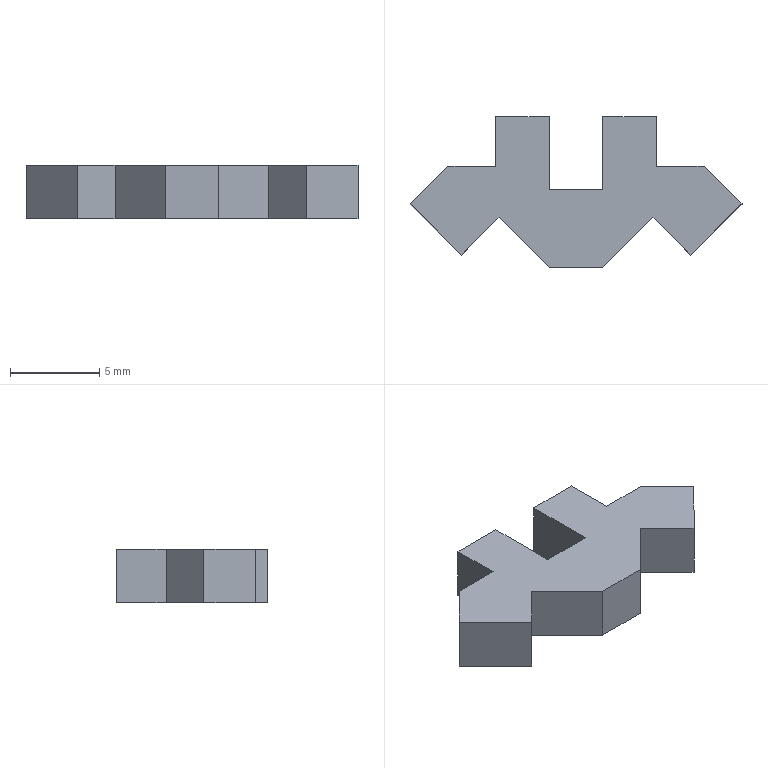Part | SolidWorks | features BaseBody 1 | 1 solid | 20 faces | box 18.567 x 8.438 x 3 mm | volume 257.816 mm3 | plane 20
STEP:
#1=CARTESIAN_POINT('',(-32.996,6.652,-1.5));
#2=VERTEX_POINT('',#1);
#3=CARTESIAN_POINT('',(-35.116,8.77,-1.5));
#4=VERTEX_POINT('',#3);
#5=CARTESIAN_POINT('',(-35.116,8.77,-1.5));
#6=DIRECTION('',(-0.7074,0.7068,0.));
#7=VECTOR('',#6,1000.);
#8=LINE('',#5,#7);
#9=EDGE_CURVE('',#2,#4,#8,.T.);
#10=ORIENTED_EDGE('',*,*,#9,.F.);
#11=CARTESIAN_POINT('',(-35.854,3.792,-1.5));
#12=VERTEX_POINT('',#11);
#13=CARTESIAN_POINT('',(-32.996,6.652,-1.5));
#14=DIRECTION('',(0.7068,0.7074,0.));
#15=VECTOR('',#14,1000.);
#16=LINE('',#13,#15);
#17=EDGE_CURVE('',#12,#2,#16,.T.);
#18=ORIENTED_EDGE('',*,*,#17,.F.);
#19=CARTESIAN_POINT('',(-37.974,5.912,-1.5));
#20=VERTEX_POINT('',#19);
#21=CARTESIAN_POINT('',(-35.854,3.792,-1.5));
#22=DIRECTION('',(0.707,-0.7072,0.));
#23=VECTOR('',#22,1000.);
#24=LINE('',#21,#23);
#25=EDGE_CURVE('',#20,#12,#24,.T.);
#26=ORIENTED_EDGE('',*,*,#25,.F.);
#27=CARTESIAN_POINT('',(-40.782,3.103,-1.5));
#28=VERTEX_POINT('',#27);
#29=CARTESIAN_POINT('',(-37.974,5.912,-1.5));
#30=DIRECTION('',(0.707,0.7072,0.));
#31=VECTOR('',#30,1000.);
#32=LINE('',#29,#31);
#33=EDGE_CURVE('',#28,#20,#32,.T.);
#34=ORIENTED_EDGE('',*,*,#33,.F.);
#35=CARTESIAN_POINT('',(-43.778,3.103,-1.5));
#36=VERTEX_POINT('',#35);
#37=CARTESIAN_POINT('',(-40.782,3.103,-1.5));
#38=DIRECTION('',(1.,0.,0.));
#39=VECTOR('',#38,1000.);
#40=LINE('',#37,#39);
#41=EDGE_CURVE('',#36,#28,#40,.T.);
#42=ORIENTED_EDGE('',*,*,#41,.F.);
#43=CARTESIAN_POINT('',(-46.585,5.913,-1.5));
#44=VERTEX_POINT('',#43);
#45=CARTESIAN_POINT('',(-43.778,3.103,-1.5));
#46=DIRECTION('',(0.7067,-0.7075,0.));
#47=VECTOR('',#46,1000.);
#48=LINE('',#45,#47);
#49=EDGE_CURVE('',#44,#36,#48,.T.);
#50=ORIENTED_EDGE('',*,*,#49,.F.);
#51=CARTESIAN_POINT('',(-48.705,3.792,-1.5));
#52=VERTEX_POINT('',#51);
#53=CARTESIAN_POINT('',(-46.585,5.913,-1.5));
#54=DIRECTION('',(0.707,0.7072,0.));
#55=VECTOR('',#54,1000.);
#56=LINE('',#53,#55);
#57=EDGE_CURVE('',#52,#44,#56,.T.);
#58=ORIENTED_EDGE('',*,*,#57,.F.);
#59=CARTESIAN_POINT('',(-51.564,6.652,-1.5));
#60=VERTEX_POINT('',#59);
#61=CARTESIAN_POINT('',(-48.705,3.792,-1.5));
#62=DIRECTION('',(0.7068,-0.7074,0.));
#63=VECTOR('',#62,1000.);
#64=LINE('',#61,#63);
#65=EDGE_CURVE('',#60,#52,#64,.T.);
#66=ORIENTED_EDGE('',*,*,#65,.F.);
#67=CARTESIAN_POINT('',(-49.444,8.77,-1.5));
#68=VERTEX_POINT('',#67);
#69=CARTESIAN_POINT('',(-51.564,6.652,-1.5));
#70=DIRECTION('',(-0.7074,-0.7068,0.));
#71=VECTOR('',#70,1000.);
#72=LINE('',#69,#71);
#73=EDGE_CURVE('',#68,#60,#72,.T.);
#74=ORIENTED_EDGE('',*,*,#73,.F.);
#75=CARTESIAN_POINT('',(-46.773,8.77,-1.5));
#76=VERTEX_POINT('',#75);
#77=CARTESIAN_POINT('',(-49.444,8.77,-1.5));
#78=DIRECTION('',(-1.,0.,0.));
#79=VECTOR('',#78,1000.);
#80=LINE('',#77,#79);
#81=EDGE_CURVE('',#76,#68,#80,.T.);
#82=ORIENTED_EDGE('',*,*,#81,.F.);
#83=CARTESIAN_POINT('',(-46.773,11.54,-1.5));
#84=VERTEX_POINT('',#83);
#85=CARTESIAN_POINT('',(-46.773,8.77,-1.5));
#86=DIRECTION('',(0.,-1.,0.));
#87=VECTOR('',#86,1000.);
#88=LINE('',#85,#87);
#89=EDGE_CURVE('',#84,#76,#88,.T.);
#90=ORIENTED_EDGE('',*,*,#89,.F.);
#91=CARTESIAN_POINT('',(-43.778,11.54,-1.5));
#92=VERTEX_POINT('',#91);
#93=CARTESIAN_POINT('',(-46.773,11.54,-1.5));
#94=DIRECTION('',(-1.,0.,0.));
#95=VECTOR('',#94,1000.);
#96=LINE('',#93,#95);
#97=EDGE_CURVE('',#92,#84,#96,.T.);
#98=ORIENTED_EDGE('',*,*,#97,.F.);
#99=CARTESIAN_POINT('',(-43.778,7.443,-1.5));
#100=VERTEX_POINT('',#99);
#101=CARTESIAN_POINT('',(-43.778,11.54,-1.5));
#102=DIRECTION('',(0.,1.,0.));
#103=VECTOR('',#102,1000.);
#104=LINE('',#101,#103);
#105=EDGE_CURVE('',#100,#92,#104,.T.);
#106=ORIENTED_EDGE('',*,*,#105,.F.);
#107=CARTESIAN_POINT('',(-40.782,7.443,-1.5));
#108=VERTEX_POINT('',#107);
#109=CARTESIAN_POINT('',(-43.778,7.443,-1.5));
#110=DIRECTION('',(-1.,0.,0.));
#111=VECTOR('',#110,1000.);
#112=LINE('',#109,#111);
#113=EDGE_CURVE('',#108,#100,#112,.T.);
#114=ORIENTED_EDGE('',*,*,#113,.F.);
#115=CARTESIAN_POINT('',(-40.782,11.54,-1.5));
#116=VERTEX_POINT('',#115);
#117=CARTESIAN_POINT('',(-40.782,7.443,-1.5));
#118=DIRECTION('',(0.,-1.,0.));
#119=VECTOR('',#118,1000.);
#120=LINE('',#117,#119);
#121=EDGE_CURVE('',#116,#108,#120,.T.);
#122=ORIENTED_EDGE('',*,*,#121,.F.);
#123=CARTESIAN_POINT('',(-37.786,11.54,-1.5));
#124=VERTEX_POINT('',#123);
#125=CARTESIAN_POINT('',(-40.782,11.54,-1.5));
#126=DIRECTION('',(-1.,0.,0.));
#127=VECTOR('',#126,1000.);
#128=LINE('',#125,#127);
#129=EDGE_CURVE('',#124,#116,#128,.T.);
#130=ORIENTED_EDGE('',*,*,#129,.F.);
#131=CARTESIAN_POINT('',(-37.786,8.77,-1.5));
#132=VERTEX_POINT('',#131);
#133=CARTESIAN_POINT('',(-37.786,11.54,-1.5));
#134=DIRECTION('',(0.,1.,0.));
#135=VECTOR('',#134,1000.);
#136=LINE('',#133,#135);
#137=EDGE_CURVE('',#132,#124,#136,.T.);
#138=ORIENTED_EDGE('',*,*,#137,.F.);
#139=CARTESIAN_POINT('',(-37.786,8.77,-1.5));
#140=DIRECTION('',(-1.,0.,0.));
#141=VECTOR('',#140,1000.);
#142=LINE('',#139,#141);
#143=EDGE_CURVE('',#4,#132,#142,.T.);
#144=ORIENTED_EDGE('',*,*,#143,.F.);
#145=EDGE_LOOP('',(#10,#18,#26,#34,#42,#50,#58,#66,#74,#82,#90,#98,#106,#114,#122,#130,#138,#144));
#146=FACE_OUTER_BOUND('',#145,.T.);
#147=CARTESIAN_POINT('',(0.,0.,-1.5));
#148=DIRECTION('',(0.,0.,-1.));
#149=DIRECTION('',(0.,-1.,0.));
#150=AXIS2_PLACEMENT_3D('',#147,#148,#149);
#151=PLANE('',#150);
#152=ADVANCED_FACE('',(#146),#151,.T.);
#153=CARTESIAN_POINT('',(-32.996,6.652,1.5));
#154=VERTEX_POINT('',#153);
#155=CARTESIAN_POINT('',(-35.116,8.77,1.5));
#156=VERTEX_POINT('',#155);
#157=CARTESIAN_POINT('',(-35.116,8.77,1.5));
#158=DIRECTION('',(-0.7074,0.7068,0.));
#159=VECTOR('',#158,1000.);
#160=LINE('',#157,#159);
#161=EDGE_CURVE('',#154,#156,#160,.T.);
#162=ORIENTED_EDGE('',*,*,#161,.T.);
#163=CARTESIAN_POINT('',(-37.786,8.77,1.5));
#164=VERTEX_POINT('',#163);
#165=CARTESIAN_POINT('',(-37.786,8.77,1.5));
#166=DIRECTION('',(-1.,0.,0.));
#167=VECTOR('',#166,1000.);
#168=LINE('',#165,#167);
#169=EDGE_CURVE('',#156,#164,#168,.T.);
#170=ORIENTED_EDGE('',*,*,#169,.T.);
#171=CARTESIAN_POINT('',(-37.786,11.54,1.5));
#172=VERTEX_POINT('',#171);
#173=CARTESIAN_POINT('',(-37.786,11.54,1.5));
#174=DIRECTION('',(0.,1.,0.));
#175=VECTOR('',#174,1000.);
#176=LINE('',#173,#175);
#177=EDGE_CURVE('',#164,#172,#176,.T.);
#178=ORIENTED_EDGE('',*,*,#177,.T.);
#179=CARTESIAN_POINT('',(-40.782,11.54,1.5));
#180=VERTEX_POINT('',#179);
#181=CARTESIAN_POINT('',(-40.782,11.54,1.5));
#182=DIRECTION('',(-1.,0.,0.));
#183=VECTOR('',#182,1000.);
#184=LINE('',#181,#183);
#185=EDGE_CURVE('',#172,#180,#184,.T.);
#186=ORIENTED_EDGE('',*,*,#185,.T.);
#187=CARTESIAN_POINT('',(-40.782,7.443,1.5));
#188=VERTEX_POINT('',#187);
#189=CARTESIAN_POINT('',(-40.782,7.443,1.5));
#190=DIRECTION('',(0.,-1.,0.));
#191=VECTOR('',#190,1000.);
#192=LINE('',#189,#191);
#193=EDGE_CURVE('',#180,#188,#192,.T.);
#194=ORIENTED_EDGE('',*,*,#193,.T.);
#195=CARTESIAN_POINT('',(-43.778,7.443,1.5));
#196=VERTEX_POINT('',#195);
#197=CARTESIAN_POINT('',(-43.778,7.443,1.5));
#198=DIRECTION('',(-1.,0.,0.));
#199=VECTOR('',#198,1000.);
#200=LINE('',#197,#199);
#201=EDGE_CURVE('',#188,#196,#200,.T.);
#202=ORIENTED_EDGE('',*,*,#201,.T.);
#203=CARTESIAN_POINT('',(-43.778,11.54,1.5));
#204=VERTEX_POINT('',#203);
#205=CARTESIAN_POINT('',(-43.778,11.54,1.5));
#206=DIRECTION('',(0.,1.,0.));
#207=VECTOR('',#206,1000.);
#208=LINE('',#205,#207);
#209=EDGE_CURVE('',#196,#204,#208,.T.);
#210=ORIENTED_EDGE('',*,*,#209,.T.);
#211=CARTESIAN_POINT('',(-46.773,11.54,1.5));
#212=VERTEX_POINT('',#211);
#213=CARTESIAN_POINT('',(-46.773,11.54,1.5));
#214=DIRECTION('',(-1.,0.,0.));
#215=VECTOR('',#214,1000.);
#216=LINE('',#213,#215);
#217=EDGE_CURVE('',#204,#212,#216,.T.);
#218=ORIENTED_EDGE('',*,*,#217,.T.);
#219=CARTESIAN_POINT('',(-46.773,8.77,1.5));
#220=VERTEX_POINT('',#219);
#221=CARTESIAN_POINT('',(-46.773,8.77,1.5));
#222=DIRECTION('',(0.,-1.,0.));
#223=VECTOR('',#222,1000.);
#224=LINE('',#221,#223);
#225=EDGE_CURVE('',#212,#220,#224,.T.);
#226=ORIENTED_EDGE('',*,*,#225,.T.);
#227=CARTESIAN_POINT('',(-49.444,8.77,1.5));
#228=VERTEX_POINT('',#227);
#229=CARTESIAN_POINT('',(-49.444,8.77,1.5));
#230=DIRECTION('',(-1.,0.,0.));
#231=VECTOR('',#230,1000.);
#232=LINE('',#229,#231);
#233=EDGE_CURVE('',#220,#228,#232,.T.);
#234=ORIENTED_EDGE('',*,*,#233,.T.);
#235=CARTESIAN_POINT('',(-51.564,6.652,1.5));
#236=VERTEX_POINT('',#235);
#237=CARTESIAN_POINT('',(-51.564,6.652,1.5));
#238=DIRECTION('',(-0.7074,-0.7068,0.));
#239=VECTOR('',#238,1000.);
#240=LINE('',#237,#239);
#241=EDGE_CURVE('',#228,#236,#240,.T.);
#242=ORIENTED_EDGE('',*,*,#241,.T.);
#243=CARTESIAN_POINT('',(-48.705,3.792,1.5));
#244=VERTEX_POINT('',#243);
#245=CARTESIAN_POINT('',(-48.705,3.792,1.5));
#246=DIRECTION('',(0.7068,-0.7074,0.));
#247=VECTOR('',#246,1000.);
#248=LINE('',#245,#247);
#249=EDGE_CURVE('',#236,#244,#248,.T.);
#250=ORIENTED_EDGE('',*,*,#249,.T.);
#251=CARTESIAN_POINT('',(-46.585,5.913,1.5));
#252=VERTEX_POINT('',#251);
#253=CARTESIAN_POINT('',(-46.585,5.913,1.5));
#254=DIRECTION('',(0.707,0.7072,0.));
#255=VECTOR('',#254,1000.);
#256=LINE('',#253,#255);
#257=EDGE_CURVE('',#244,#252,#256,.T.);
#258=ORIENTED_EDGE('',*,*,#257,.T.);
#259=CARTESIAN_POINT('',(-43.778,3.103,1.5));
#260=VERTEX_POINT('',#259);
#261=CARTESIAN_POINT('',(-43.778,3.103,1.5));
#262=DIRECTION('',(0.7067,-0.7075,0.));
#263=VECTOR('',#262,1000.);
#264=LINE('',#261,#263);
#265=EDGE_CURVE('',#252,#260,#264,.T.);
#266=ORIENTED_EDGE('',*,*,#265,.T.);
#267=CARTESIAN_POINT('',(-40.782,3.103,1.5));
#268=VERTEX_POINT('',#267);
#269=CARTESIAN_POINT('',(-40.782,3.103,1.5));
#270=DIRECTION('',(1.,0.,0.));
#271=VECTOR('',#270,1000.);
#272=LINE('',#269,#271);
#273=EDGE_CURVE('',#260,#268,#272,.T.);
#274=ORIENTED_EDGE('',*,*,#273,.T.);
#275=CARTESIAN_POINT('',(-37.974,5.912,1.5));
#276=VERTEX_POINT('',#275);
#277=CARTESIAN_POINT('',(-37.974,5.912,1.5));
#278=DIRECTION('',(0.707,0.7072,0.));
#279=VECTOR('',#278,1000.);
#280=LINE('',#277,#279);
#281=EDGE_CURVE('',#268,#276,#280,.T.);
#282=ORIENTED_EDGE('',*,*,#281,.T.);
#283=CARTESIAN_POINT('',(-35.854,3.792,1.5));
#284=VERTEX_POINT('',#283);
#285=CARTESIAN_POINT('',(-35.854,3.792,1.5));
#286=DIRECTION('',(0.707,-0.7072,0.));
#287=VECTOR('',#286,1000.);
#288=LINE('',#285,#287);
#289=EDGE_CURVE('',#276,#284,#288,.T.);
#290=ORIENTED_EDGE('',*,*,#289,.T.);
#291=CARTESIAN_POINT('',(-32.996,6.652,1.5));
#292=DIRECTION('',(0.7068,0.7074,0.));
#293=VECTOR('',#292,1000.);
#294=LINE('',#291,#293);
#295=EDGE_CURVE('',#284,#154,#294,.T.);
#296=ORIENTED_EDGE('',*,*,#295,.T.);
#297=EDGE_LOOP('',(#162,#170,#178,#186,#194,#202,#210,#218,#226,#234,#242,#250,#258,#266,#274,#282,#290,#296));
#298=FACE_OUTER_BOUND('',#297,.T.);
#299=CARTESIAN_POINT('',(0.,0.,1.5));
#300=DIRECTION('',(0.,0.,-1.));
#301=DIRECTION('',(0.,-1.,0.));
#302=AXIS2_PLACEMENT_3D('',#299,#300,#301);
#303=PLANE('',#302);
#304=ADVANCED_FACE('',(#298),#303,.F.);
#305=ORIENTED_EDGE('',*,*,#17,.T.);
#306=CARTESIAN_POINT('',(-32.996,6.652,1.5));
#307=DIRECTION('',(0.,0.,-1.));
#308=VECTOR('',#307,1000.);
#309=LINE('',#306,#308);
#310=EDGE_CURVE('',#154,#2,#309,.T.);
#311=ORIENTED_EDGE('',*,*,#310,.F.);
#312=ORIENTED_EDGE('',*,*,#295,.F.);
#313=CARTESIAN_POINT('',(-35.854,3.792,1.5));
#314=DIRECTION('',(0.,0.,-1.));
#315=VECTOR('',#314,1000.);
#316=LINE('',#313,#315);
#317=EDGE_CURVE('',#284,#12,#316,.T.);
#318=ORIENTED_EDGE('',*,*,#317,.T.);
#319=EDGE_LOOP('',(#305,#311,#312,#318));
#320=FACE_OUTER_BOUND('',#319,.T.);
#321=CARTESIAN_POINT('',(-32.996,6.652,1.5));
#322=DIRECTION('',(-0.7074,0.7068,0.));
#323=DIRECTION('',(0.,0.,1.));
#324=AXIS2_PLACEMENT_3D('',#321,#322,#323);
#325=PLANE('',#324);
#326=ADVANCED_FACE('',(#320),#325,.F.);
#327=ORIENTED_EDGE('',*,*,#25,.T.);
#328=ORIENTED_EDGE('',*,*,#317,.F.);
#329=ORIENTED_EDGE('',*,*,#289,.F.);
#330=CARTESIAN_POINT('',(-37.974,5.912,1.5));
#331=DIRECTION('',(0.,0.,-1.));
#332=VECTOR('',#331,1000.);
#333=LINE('',#330,#332);
#334=EDGE_CURVE('',#276,#20,#333,.T.);
#335=ORIENTED_EDGE('',*,*,#334,.T.);
#336=EDGE_LOOP('',(#327,#328,#329,#335));
#337=FACE_OUTER_BOUND('',#336,.T.);
#338=CARTESIAN_POINT('',(-35.854,3.792,1.5));
#339=DIRECTION('',(0.7072,0.707,0.));
#340=DIRECTION('',(0.,0.,-1.));
#341=AXIS2_PLACEMENT_3D('',#338,#339,#340);
#342=PLANE('',#341);
#343=ADVANCED_FACE('',(#337),#342,.F.);
#344=ORIENTED_EDGE('',*,*,#33,.T.);
#345=ORIENTED_EDGE('',*,*,#334,.F.);
#346=ORIENTED_EDGE('',*,*,#281,.F.);
#347=CARTESIAN_POINT('',(-40.782,3.103,1.5));
#348=DIRECTION('',(0.,0.,-1.));
#349=VECTOR('',#348,1000.);
#350=LINE('',#347,#349);
#351=EDGE_CURVE('',#268,#28,#350,.T.);
#352=ORIENTED_EDGE('',*,*,#351,.T.);
#353=EDGE_LOOP('',(#344,#345,#346,#352));
#354=FACE_OUTER_BOUND('',#353,.T.);
#355=CARTESIAN_POINT('',(-37.974,5.912,1.5));
#356=DIRECTION('',(-0.7072,0.707,0.));
#357=DIRECTION('',(0.,0.,1.));
#358=AXIS2_PLACEMENT_3D('',#355,#356,#357);
#359=PLANE('',#358);
#360=ADVANCED_FACE('',(#354),#359,.F.);
#361=ORIENTED_EDGE('',*,*,#41,.T.);
#362=ORIENTED_EDGE('',*,*,#351,.F.);
#363=ORIENTED_EDGE('',*,*,#273,.F.);
#364=CARTESIAN_POINT('',(-43.778,3.103,1.5));
#365=DIRECTION('',(0.,0.,-1.));
#366=VECTOR('',#365,1000.);
#367=LINE('',#364,#366);
#368=EDGE_CURVE('',#260,#36,#367,.T.);
#369=ORIENTED_EDGE('',*,*,#368,.T.);
#370=EDGE_LOOP('',(#361,#362,#363,#369));
#371=FACE_OUTER_BOUND('',#370,.T.);
#372=CARTESIAN_POINT('',(-40.782,3.103,1.5));
#373=DIRECTION('',(0.,1.,0.));
#374=DIRECTION('',(1.,0.,0.));
#375=AXIS2_PLACEMENT_3D('',#372,#373,#374);
#376=PLANE('',#375);
#377=ADVANCED_FACE('',(#371),#376,.F.);
#378=ORIENTED_EDGE('',*,*,#49,.T.);
#379=ORIENTED_EDGE('',*,*,#368,.F.);
#380=ORIENTED_EDGE('',*,*,#265,.F.);
#381=CARTESIAN_POINT('',(-46.585,5.913,1.5));
#382=DIRECTION('',(0.,0.,-1.));
#383=VECTOR('',#382,1000.);
#384=LINE('',#381,#383);
#385=EDGE_CURVE('',#252,#44,#384,.T.);
#386=ORIENTED_EDGE('',*,*,#385,.T.);
#387=EDGE_LOOP('',(#378,#379,#380,#386));
#388=FACE_OUTER_BOUND('',#387,.T.);
#389=CARTESIAN_POINT('',(-43.778,3.103,1.5));
#390=DIRECTION('',(0.7075,0.7067,0.));
#391=DIRECTION('',(0.,0.,-1.));
#392=AXIS2_PLACEMENT_3D('',#389,#390,#391);
#393=PLANE('',#392);
#394=ADVANCED_FACE('',(#388),#393,.F.);
#395=ORIENTED_EDGE('',*,*,#57,.T.);
#396=ORIENTED_EDGE('',*,*,#385,.F.);
#397=ORIENTED_EDGE('',*,*,#257,.F.);
#398=CARTESIAN_POINT('',(-48.705,3.792,1.5));
#399=DIRECTION('',(0.,0.,-1.));
#400=VECTOR('',#399,1000.);
#401=LINE('',#398,#400);
#402=EDGE_CURVE('',#244,#52,#401,.T.);
#403=ORIENTED_EDGE('',*,*,#402,.T.);
#404=EDGE_LOOP('',(#395,#396,#397,#403));
#405=FACE_OUTER_BOUND('',#404,.T.);
#406=CARTESIAN_POINT('',(-46.585,5.913,1.5));
#407=DIRECTION('',(-0.7072,0.707,0.));
#408=DIRECTION('',(0.,0.,1.));
#409=AXIS2_PLACEMENT_3D('',#406,#407,#408);
#410=PLANE('',#409);
#411=ADVANCED_FACE('',(#405),#410,.F.);
#412=ORIENTED_EDGE('',*,*,#65,.T.);
#413=ORIENTED_EDGE('',*,*,#402,.F.);
#414=ORIENTED_EDGE('',*,*,#249,.F.);
#415=CARTESIAN_POINT('',(-51.564,6.652,1.5));
#416=DIRECTION('',(0.,0.,-1.));
#417=VECTOR('',#416,1000.);
#418=LINE('',#415,#417);
#419=EDGE_CURVE('',#236,#60,#418,.T.);
#420=ORIENTED_EDGE('',*,*,#419,.T.);
#421=EDGE_LOOP('',(#412,#413,#414,#420));
#422=FACE_OUTER_BOUND('',#421,.T.);
#423=CARTESIAN_POINT('',(-48.705,3.792,1.5));
#424=DIRECTION('',(0.7074,0.7068,0.));
#425=DIRECTION('',(0.,0.,-1.));
#426=AXIS2_PLACEMENT_3D('',#423,#424,#425);
#427=PLANE('',#426);
#428=ADVANCED_FACE('',(#422),#427,.F.);
#429=ORIENTED_EDGE('',*,*,#73,.T.);
#430=ORIENTED_EDGE('',*,*,#419,.F.);
#431=ORIENTED_EDGE('',*,*,#241,.F.);
#432=CARTESIAN_POINT('',(-49.444,8.77,1.5));
#433=DIRECTION('',(0.,0.,-1.));
#434=VECTOR('',#433,1000.);
#435=LINE('',#432,#434);
#436=EDGE_CURVE('',#228,#68,#435,.T.);
#437=ORIENTED_EDGE('',*,*,#436,.T.);
#438=EDGE_LOOP('',(#429,#430,#431,#437));
#439=FACE_OUTER_BOUND('',#438,.T.);
#440=CARTESIAN_POINT('',(-51.564,6.652,1.5));
#441=DIRECTION('',(0.7068,-0.7074,0.));
#442=DIRECTION('',(0.,0.,-1.));
#443=AXIS2_PLACEMENT_3D('',#440,#441,#442);
#444=PLANE('',#443);
#445=ADVANCED_FACE('',(#439),#444,.F.);
#446=ORIENTED_EDGE('',*,*,#81,.T.);
#447=ORIENTED_EDGE('',*,*,#436,.F.);
#448=ORIENTED_EDGE('',*,*,#233,.F.);
#449=CARTESIAN_POINT('',(-46.773,8.77,1.5));
#450=DIRECTION('',(0.,0.,-1.));
#451=VECTOR('',#450,1000.);
#452=LINE('',#449,#451);
#453=EDGE_CURVE('',#220,#76,#452,.T.);
#454=ORIENTED_EDGE('',*,*,#453,.T.);
#455=EDGE_LOOP('',(#446,#447,#448,#454));
#456=FACE_OUTER_BOUND('',#455,.T.);
#457=CARTESIAN_POINT('',(-49.444,8.77,1.5));
#458=DIRECTION('',(0.,-1.,0.));
#459=DIRECTION('',(0.,0.,-1.));
#460=AXIS2_PLACEMENT_3D('',#457,#458,#459);
#461=PLANE('',#460);
#462=ADVANCED_FACE('',(#456),#461,.F.);
#463=ORIENTED_EDGE('',*,*,#89,.T.);
#464=ORIENTED_EDGE('',*,*,#453,.F.);
#465=ORIENTED_EDGE('',*,*,#225,.F.);
#466=CARTESIAN_POINT('',(-46.773,11.54,1.5));
#467=DIRECTION('',(0.,0.,-1.));
#468=VECTOR('',#467,1000.);
#469=LINE('',#466,#468);
#470=EDGE_CURVE('',#212,#84,#469,.T.);
#471=ORIENTED_EDGE('',*,*,#470,.T.);
#472=EDGE_LOOP('',(#463,#464,#465,#471));
#473=FACE_OUTER_BOUND('',#472,.T.);
#474=CARTESIAN_POINT('',(-46.773,8.77,1.5));
#475=DIRECTION('',(1.,0.,0.));
#476=DIRECTION('',(0.,1.,0.));
#477=AXIS2_PLACEMENT_3D('',#474,#475,#476);
#478=PLANE('',#477);
#479=ADVANCED_FACE('',(#473),#478,.F.);
#480=ORIENTED_EDGE('',*,*,#97,.T.);
#481=ORIENTED_EDGE('',*,*,#470,.F.);
#482=ORIENTED_EDGE('',*,*,#217,.F.);
#483=CARTESIAN_POINT('',(-43.778,11.54,1.5));
#484=DIRECTION('',(0.,0.,-1.));
#485=VECTOR('',#484,1000.);
#486=LINE('',#483,#485);
#487=EDGE_CURVE('',#204,#92,#486,.T.);
#488=ORIENTED_EDGE('',*,*,#487,.T.);
#489=EDGE_LOOP('',(#480,#481,#482,#488));
#490=FACE_OUTER_BOUND('',#489,.T.);
#491=CARTESIAN_POINT('',(-46.773,11.54,1.5));
#492=DIRECTION('',(0.,-1.,0.));
#493=DIRECTION('',(0.,0.,-1.));
#494=AXIS2_PLACEMENT_3D('',#491,#492,#493);
#495=PLANE('',#494);
#496=ADVANCED_FACE('',(#490),#495,.F.);
#497=ORIENTED_EDGE('',*,*,#105,.T.);
#498=ORIENTED_EDGE('',*,*,#487,.F.);
#499=ORIENTED_EDGE('',*,*,#209,.F.);
#500=CARTESIAN_POINT('',(-43.778,7.443,1.5));
#501=DIRECTION('',(0.,0.,-1.));
#502=VECTOR('',#501,1000.);
#503=LINE('',#500,#502);
#504=EDGE_CURVE('',#196,#100,#503,.T.);
#505=ORIENTED_EDGE('',*,*,#504,.T.);
#506=EDGE_LOOP('',(#497,#498,#499,#505));
#507=FACE_OUTER_BOUND('',#506,.T.);
#508=CARTESIAN_POINT('',(-43.778,11.54,1.5));
#509=DIRECTION('',(-1.,0.,0.));
#510=DIRECTION('',(0.,0.,1.));
#511=AXIS2_PLACEMENT_3D('',#508,#509,#510);
#512=PLANE('',#511);
#513=ADVANCED_FACE('',(#507),#512,.F.);
#514=ORIENTED_EDGE('',*,*,#113,.T.);
#515=ORIENTED_EDGE('',*,*,#504,.F.);
#516=ORIENTED_EDGE('',*,*,#201,.F.);
#517=CARTESIAN_POINT('',(-40.782,7.443,1.5));
#518=DIRECTION('',(0.,0.,-1.));
#519=VECTOR('',#518,1000.);
#520=LINE('',#517,#519);
#521=EDGE_CURVE('',#188,#108,#520,.T.);
#522=ORIENTED_EDGE('',*,*,#521,.T.);
#523=EDGE_LOOP('',(#514,#515,#516,#522));
#524=FACE_OUTER_BOUND('',#523,.T.);
#525=CARTESIAN_POINT('',(-43.778,7.443,1.5));
#526=DIRECTION('',(0.,-1.,0.));
#527=DIRECTION('',(0.,0.,-1.));
#528=AXIS2_PLACEMENT_3D('',#525,#526,#527);
#529=PLANE('',#528);
#530=ADVANCED_FACE('',(#524),#529,.F.);
#531=ORIENTED_EDGE('',*,*,#121,.T.);
#532=ORIENTED_EDGE('',*,*,#521,.F.);
#533=ORIENTED_EDGE('',*,*,#193,.F.);
#534=CARTESIAN_POINT('',(-40.782,11.54,1.5));
#535=DIRECTION('',(0.,0.,-1.));
#536=VECTOR('',#535,1000.);
#537=LINE('',#534,#536);
#538=EDGE_CURVE('',#180,#116,#537,.T.);
#539=ORIENTED_EDGE('',*,*,#538,.T.);
#540=EDGE_LOOP('',(#531,#532,#533,#539));
#541=FACE_OUTER_BOUND('',#540,.T.);
#542=CARTESIAN_POINT('',(-40.782,7.443,1.5));
#543=DIRECTION('',(1.,0.,0.));
#544=DIRECTION('',(0.,1.,0.));
#545=AXIS2_PLACEMENT_3D('',#542,#543,#544);
#546=PLANE('',#545);
#547=ADVANCED_FACE('',(#541),#546,.F.);
#548=ORIENTED_EDGE('',*,*,#129,.T.);
#549=ORIENTED_EDGE('',*,*,#538,.F.);
#550=ORIENTED_EDGE('',*,*,#185,.F.);
#551=CARTESIAN_POINT('',(-37.786,11.54,1.5));
#552=DIRECTION('',(0.,0.,-1.));
#553=VECTOR('',#552,1000.);
#554=LINE('',#551,#553);
#555=EDGE_CURVE('',#172,#124,#554,.T.);
#556=ORIENTED_EDGE('',*,*,#555,.T.);
#557=EDGE_LOOP('',(#548,#549,#550,#556));
#558=FACE_OUTER_BOUND('',#557,.T.);
#559=CARTESIAN_POINT('',(-40.782,11.54,1.5));
#560=DIRECTION('',(0.,-1.,0.));
#561=DIRECTION('',(0.,0.,-1.));
#562=AXIS2_PLACEMENT_3D('',#559,#560,#561);
#563=PLANE('',#562);
#564=ADVANCED_FACE('',(#558),#563,.F.);
#565=ORIENTED_EDGE('',*,*,#137,.T.);
#566=ORIENTED_EDGE('',*,*,#555,.F.);
#567=ORIENTED_EDGE('',*,*,#177,.F.);
#568=CARTESIAN_POINT('',(-37.786,8.77,1.5));
#569=DIRECTION('',(0.,0.,-1.));
#570=VECTOR('',#569,1000.);
#571=LINE('',#568,#570);
#572=EDGE_CURVE('',#164,#132,#571,.T.);
#573=ORIENTED_EDGE('',*,*,#572,.T.);
#574=EDGE_LOOP('',(#565,#566,#567,#573));
#575=FACE_OUTER_BOUND('',#574,.T.);
#576=CARTESIAN_POINT('',(-37.786,11.54,1.5));
#577=DIRECTION('',(-1.,0.,0.));
#578=DIRECTION('',(0.,0.,1.));
#579=AXIS2_PLACEMENT_3D('',#576,#577,#578);
#580=PLANE('',#579);
#581=ADVANCED_FACE('',(#575),#580,.F.);
#582=ORIENTED_EDGE('',*,*,#143,.T.);
#583=ORIENTED_EDGE('',*,*,#572,.F.);
#584=ORIENTED_EDGE('',*,*,#169,.F.);
#585=CARTESIAN_POINT('',(-35.116,8.77,1.5));
#586=DIRECTION('',(0.,0.,-1.));
#587=VECTOR('',#586,1000.);
#588=LINE('',#585,#587);
#589=EDGE_CURVE('',#156,#4,#588,.T.);
#590=ORIENTED_EDGE('',*,*,#589,.T.);
#591=EDGE_LOOP('',(#582,#583,#584,#590));
#592=FACE_OUTER_BOUND('',#591,.T.);
#593=CARTESIAN_POINT('',(-37.786,8.77,1.5));
#594=DIRECTION('',(0.,-1.,0.));
#595=DIRECTION('',(0.,0.,-1.));
#596=AXIS2_PLACEMENT_3D('',#593,#594,#595);
#597=PLANE('',#596);
#598=ADVANCED_FACE('',(#592),#597,.F.);
#599=ORIENTED_EDGE('',*,*,#9,.T.);
#600=ORIENTED_EDGE('',*,*,#589,.F.);
#601=ORIENTED_EDGE('',*,*,#161,.F.);
#602=ORIENTED_EDGE('',*,*,#310,.T.);
#603=EDGE_LOOP('',(#599,#600,#601,#602));
#604=FACE_OUTER_BOUND('',#603,.T.);
#605=CARTESIAN_POINT('',(-35.116,8.77,1.5));
#606=DIRECTION('',(-0.7068,-0.7074,0.));
#607=DIRECTION('',(-0.7074,0.7068,0.));
#608=AXIS2_PLACEMENT_3D('',#605,#606,#607);
#609=PLANE('',#608);
#610=ADVANCED_FACE('',(#604),#609,.F.);
#611=CLOSED_SHELL('',(#152,#304,#326,#343,#360,#377,#394,#411,#428,#445,#462,#479,#496,#513,#530,#547,#564,#581,#598,#610));
#612=MANIFOLD_SOLID_BREP('',#611);
#613=CARTESIAN_POINT('',(0.,0.,0.));
#614=DIRECTION('',(0.,0.,1.));
#615=DIRECTION('',(1.,0.,0.));
#616=AXIS2_PLACEMENT_3D('',#613,#614,#615);
#617=(LENGTH_UNIT()NAMED_UNIT(*)SI_UNIT(.MILLI.,.METRE.));
#618=UNCERTAINTY_MEASURE_WITH_UNIT(LENGTH_MEASURE(0.00001),#617,'','');
#619=(NAMED_UNIT(*)PLANE_ANGLE_UNIT()SI_UNIT($,.RADIAN.));
#620=(NAMED_UNIT(*)SI_UNIT($,.STERADIAN.)SOLID_ANGLE_UNIT());
#621=(GEOMETRIC_REPRESENTATION_CONTEXT(3)GLOBAL_UNCERTAINTY_ASSIGNED_CONTEXT((#618))GLOBAL_UNIT_ASSIGNED_CONTEXT((#617,#619,#620))REPRESENTATION_CONTEXT('',''));
#622=ADVANCED_BREP_SHAPE_REPRESENTATION('',(#612,#616),#621);